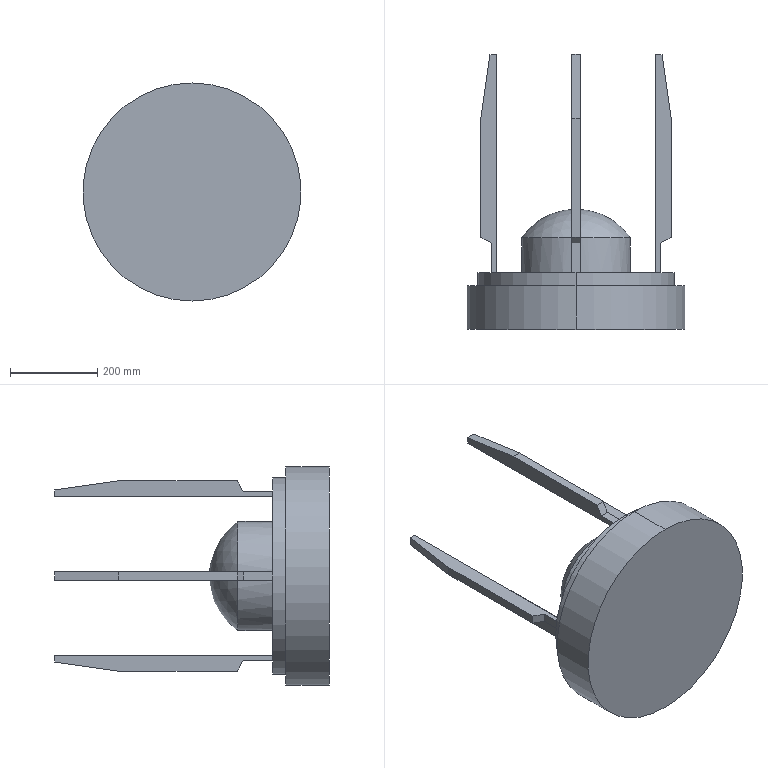Part | SolidWorks | features ICE 3, Revolution 2, CirPattern 1 | 1 solid | 43 faces | box 500 x 630 x 500 mm | volume 31254702 mm3 | plane 35 | cylinder 6 | sphere 2 | commonest cylinder face diameters 250 x2 450 x2 500 x2
STEP:
#1=CARTESIAN_POINT('',(0.,275.519,0.));
#2=VERTEX_POINT('',#1);
#3=CARTESIAN_POINT('',(125.,210.,0.));
#4=VERTEX_POINT('',#3);
#5=CARTESIAN_POINT('',(0.,123.519,0.));
#6=DIRECTION('',(0.,0.,-1.));
#7=DIRECTION('',(-1.,0.,0.));
#8=AXIS2_PLACEMENT_3D('',#5,#6,#7);
#9=CIRCLE('',#8,152.);
#10=EDGE_CURVE('',#2,#4,#9,.T.);
#11=ORIENTED_EDGE('',*,*,#10,.F.);
#12=CARTESIAN_POINT('',(-125.,210.,0.));
#13=VERTEX_POINT('',#12);
#14=CARTESIAN_POINT('',(0.,123.519,0.));
#15=DIRECTION('',(0.,0.,1.));
#16=DIRECTION('',(1.,0.,0.));
#17=AXIS2_PLACEMENT_3D('',#14,#15,#16);
#18=CIRCLE('',#17,152.);
#19=EDGE_CURVE('',#2,#13,#18,.T.);
#20=ORIENTED_EDGE('',*,*,#19,.T.);
#21=CARTESIAN_POINT('',(0.,210.,125.));
#22=VERTEX_POINT('',#21);
#23=CARTESIAN_POINT('',(0.,210.,0.));
#24=DIRECTION('',(0.,1.,0.));
#25=DIRECTION('',(0.,0.,1.));
#26=AXIS2_PLACEMENT_3D('',#23,#24,#25);
#27=CIRCLE('',#26,125.);
#28=EDGE_CURVE('',#13,#22,#27,.T.);
#29=ORIENTED_EDGE('',*,*,#28,.T.);
#30=CARTESIAN_POINT('',(0.,210.,0.));
#31=DIRECTION('',(0.,1.,0.));
#32=DIRECTION('',(0.,0.,1.));
#33=AXIS2_PLACEMENT_3D('',#30,#31,#32);
#34=CIRCLE('',#33,125.);
#35=EDGE_CURVE('',#22,#4,#34,.T.);
#36=ORIENTED_EDGE('',*,*,#35,.T.);
#37=EDGE_LOOP('',(#11,#20,#29,#36));
#38=FACE_OUTER_BOUND('',#37,.T.);
#39=CARTESIAN_POINT('',(0.,123.519,0.));
#40=DIRECTION('',(0.,0.,1.));
#41=DIRECTION('',(1.,0.,0.));
#42=AXIS2_PLACEMENT_3D('',#39,#40,#41);
#43=SPHERICAL_SURFACE('',#42,152.);
#44=ADVANCED_FACE('',(#38),#43,.T.);
#45=ORIENTED_EDGE('',*,*,#35,.F.);
#46=CARTESIAN_POINT('',(0.,130.,125.));
#47=VERTEX_POINT('',#46);
#48=CARTESIAN_POINT('',(0.,210.,125.));
#49=DIRECTION('',(0.,-1.,0.));
#50=VECTOR('',#49,1000.);
#51=LINE('',#48,#50);
#52=EDGE_CURVE('',#22,#47,#51,.T.);
#53=ORIENTED_EDGE('',*,*,#52,.T.);
#54=CARTESIAN_POINT('',(0.,130.,-125.));
#55=VERTEX_POINT('',#54);
#56=CARTESIAN_POINT('',(0.,130.,0.));
#57=DIRECTION('',(0.,1.,0.));
#58=DIRECTION('',(0.,0.,1.));
#59=AXIS2_PLACEMENT_3D('',#56,#57,#58);
#60=CIRCLE('',#59,125.);
#61=EDGE_CURVE('',#47,#55,#60,.T.);
#62=ORIENTED_EDGE('',*,*,#61,.T.);
#63=CARTESIAN_POINT('',(0.,210.,-125.));
#64=VERTEX_POINT('',#63);
#65=CARTESIAN_POINT('',(0.,210.,-125.));
#66=DIRECTION('',(0.,-1.,0.));
#67=VECTOR('',#66,1000.);
#68=LINE('',#65,#67);
#69=EDGE_CURVE('',#64,#55,#68,.T.);
#70=ORIENTED_EDGE('',*,*,#69,.F.);
#71=CARTESIAN_POINT('',(0.,210.,0.));
#72=DIRECTION('',(0.,1.,0.));
#73=DIRECTION('',(0.,0.,1.));
#74=AXIS2_PLACEMENT_3D('',#71,#72,#73);
#75=CIRCLE('',#74,125.);
#76=EDGE_CURVE('',#4,#64,#75,.T.);
#77=ORIENTED_EDGE('',*,*,#76,.F.);
#78=EDGE_LOOP('',(#45,#53,#62,#70,#77));
#79=FACE_OUTER_BOUND('',#78,.T.);
#80=CARTESIAN_POINT('',(0.,210.,0.));
#81=DIRECTION('',(0.,-1.,0.));
#82=DIRECTION('',(0.,0.,-1.));
#83=AXIS2_PLACEMENT_3D('',#80,#81,#82);
#84=CYLINDRICAL_SURFACE('',#83,125.);
#85=ADVANCED_FACE('',(#79),#84,.T.);
#86=CARTESIAN_POINT('',(0.,130.,225.));
#87=VERTEX_POINT('',#86);
#88=CARTESIAN_POINT('',(0.,130.,-225.));
#89=VERTEX_POINT('',#88);
#90=CARTESIAN_POINT('',(0.,130.,0.));
#91=DIRECTION('',(0.,1.,0.));
#92=DIRECTION('',(0.,0.,1.));
#93=AXIS2_PLACEMENT_3D('',#90,#91,#92);
#94=CIRCLE('',#93,225.);
#95=EDGE_CURVE('',#87,#89,#94,.T.);
#96=ORIENTED_EDGE('',*,*,#95,.F.);
#97=CARTESIAN_POINT('',(0.,100.,225.));
#98=VERTEX_POINT('',#97);
#99=CARTESIAN_POINT('',(0.,130.,225.));
#100=DIRECTION('',(0.,-1.,0.));
#101=VECTOR('',#100,1000.);
#102=LINE('',#99,#101);
#103=EDGE_CURVE('',#87,#98,#102,.T.);
#104=ORIENTED_EDGE('',*,*,#103,.T.);
#105=CARTESIAN_POINT('',(0.,100.,-225.));
#106=VERTEX_POINT('',#105);
#107=CARTESIAN_POINT('',(0.,100.,0.));
#108=DIRECTION('',(0.,1.,0.));
#109=DIRECTION('',(0.,0.,1.));
#110=AXIS2_PLACEMENT_3D('',#107,#108,#109);
#111=CIRCLE('',#110,225.);
#112=EDGE_CURVE('',#98,#106,#111,.T.);
#113=ORIENTED_EDGE('',*,*,#112,.T.);
#114=CARTESIAN_POINT('',(0.,130.,-225.));
#115=DIRECTION('',(0.,-1.,0.));
#116=VECTOR('',#115,1000.);
#117=LINE('',#114,#116);
#118=EDGE_CURVE('',#89,#106,#117,.T.);
#119=ORIENTED_EDGE('',*,*,#118,.F.);
#120=EDGE_LOOP('',(#96,#104,#113,#119));
#121=FACE_OUTER_BOUND('',#120,.T.);
#122=CARTESIAN_POINT('',(0.,130.,0.));
#123=DIRECTION('',(0.,-1.,0.));
#124=DIRECTION('',(0.,0.,-1.));
#125=AXIS2_PLACEMENT_3D('',#122,#123,#124);
#126=CYLINDRICAL_SURFACE('',#125,225.);
#127=ADVANCED_FACE('',(#121),#126,.T.);
#128=CARTESIAN_POINT('',(0.,100.,-250.));
#129=VERTEX_POINT('',#128);
#130=CARTESIAN_POINT('',(0.,100.,250.));
#131=VERTEX_POINT('',#130);
#132=CARTESIAN_POINT('',(0.,100.,0.));
#133=DIRECTION('',(0.,-1.,0.));
#134=DIRECTION('',(0.,0.,-1.));
#135=AXIS2_PLACEMENT_3D('',#132,#133,#134);
#136=CIRCLE('',#135,250.);
#137=EDGE_CURVE('',#129,#131,#136,.T.);
#138=ORIENTED_EDGE('',*,*,#137,.T.);
#139=CARTESIAN_POINT('',(0.,0.,250.));
#140=VERTEX_POINT('',#139);
#141=CARTESIAN_POINT('',(0.,0.,250.));
#142=DIRECTION('',(0.,-1.,0.));
#143=VECTOR('',#142,1000.);
#144=LINE('',#141,#143);
#145=EDGE_CURVE('',#131,#140,#144,.T.);
#146=ORIENTED_EDGE('',*,*,#145,.T.);
#147=CARTESIAN_POINT('',(0.,0.,-250.));
#148=VERTEX_POINT('',#147);
#149=CARTESIAN_POINT('',(0.,0.,0.));
#150=DIRECTION('',(0.,-1.,0.));
#151=DIRECTION('',(0.,0.,-1.));
#152=AXIS2_PLACEMENT_3D('',#149,#150,#151);
#153=CIRCLE('',#152,250.);
#154=EDGE_CURVE('',#148,#140,#153,.T.);
#155=ORIENTED_EDGE('',*,*,#154,.F.);
#156=CARTESIAN_POINT('',(0.,0.,-250.));
#157=DIRECTION('',(0.,-1.,0.));
#158=VECTOR('',#157,1000.);
#159=LINE('',#156,#158);
#160=EDGE_CURVE('',#129,#148,#159,.T.);
#161=ORIENTED_EDGE('',*,*,#160,.F.);
#162=EDGE_LOOP('',(#138,#146,#155,#161));
#163=FACE_OUTER_BOUND('',#162,.T.);
#164=CARTESIAN_POINT('',(0.,0.,0.));
#165=DIRECTION('',(0.,-1.,0.));
#166=DIRECTION('',(0.,0.,-1.));
#167=AXIS2_PLACEMENT_3D('',#164,#165,#166);
#168=CYLINDRICAL_SURFACE('',#167,250.);
#169=ADVANCED_FACE('',(#163),#168,.T.);
#170=ORIENTED_EDGE('',*,*,#154,.T.);
#171=CARTESIAN_POINT('',(0.,0.,0.));
#172=DIRECTION('',(0.,-1.,0.));
#173=DIRECTION('',(0.,0.,-1.));
#174=AXIS2_PLACEMENT_3D('',#171,#172,#173);
#175=CIRCLE('',#174,250.);
#176=EDGE_CURVE('',#140,#148,#175,.T.);
#177=ORIENTED_EDGE('',*,*,#176,.T.);
#178=EDGE_LOOP('',(#170,#177));
#179=FACE_OUTER_BOUND('',#178,.T.);
#180=CARTESIAN_POINT('',(250.,0.,0.));
#181=DIRECTION('',(0.,-1.,0.));
#182=DIRECTION('',(0.,0.,-1.));
#183=AXIS2_PLACEMENT_3D('',#180,#181,#182);
#184=PLANE('',#183);
#185=ADVANCED_FACE('',(#179),#184,.T.);
#186=CARTESIAN_POINT('',(0.,100.,0.));
#187=DIRECTION('',(0.,1.,0.));
#188=DIRECTION('',(0.,0.,1.));
#189=AXIS2_PLACEMENT_3D('',#186,#187,#188);
#190=CIRCLE('',#189,225.);
#191=EDGE_CURVE('',#106,#98,#190,.T.);
#192=ORIENTED_EDGE('',*,*,#191,.F.);
#193=ORIENTED_EDGE('',*,*,#112,.F.);
#194=EDGE_LOOP('',(#192,#193));
#195=FACE_BOUND('',#194,.T.);
#196=ORIENTED_EDGE('',*,*,#137,.F.);
#197=CARTESIAN_POINT('',(0.,100.,0.));
#198=DIRECTION('',(0.,-1.,0.));
#199=DIRECTION('',(0.,0.,-1.));
#200=AXIS2_PLACEMENT_3D('',#197,#198,#199);
#201=CIRCLE('',#200,250.);
#202=EDGE_CURVE('',#131,#129,#201,.T.);
#203=ORIENTED_EDGE('',*,*,#202,.F.);
#204=EDGE_LOOP('',(#196,#203));
#205=FACE_OUTER_BOUND('',#204,.T.);
#206=CARTESIAN_POINT('',(0.,100.,0.));
#207=DIRECTION('',(0.,1.,0.));
#208=DIRECTION('',(0.,0.,1.));
#209=AXIS2_PLACEMENT_3D('',#206,#207,#208);
#210=PLANE('',#209);
#211=ADVANCED_FACE('',(#195,#205),#210,.T.);
#212=ORIENTED_EDGE('',*,*,#145,.F.);
#213=ORIENTED_EDGE('',*,*,#202,.T.);
#214=ORIENTED_EDGE('',*,*,#160,.T.);
#215=ORIENTED_EDGE('',*,*,#176,.F.);
#216=EDGE_LOOP('',(#212,#213,#214,#215));
#217=FACE_OUTER_BOUND('',#216,.T.);
#218=CARTESIAN_POINT('',(0.,0.,0.));
#219=DIRECTION('',(0.,-1.,0.));
#220=DIRECTION('',(0.,0.,-1.));
#221=AXIS2_PLACEMENT_3D('',#218,#219,#220);
#222=CYLINDRICAL_SURFACE('',#221,250.);
#223=ADVANCED_FACE('',(#217),#222,.T.);
#224=ORIENTED_EDGE('',*,*,#103,.F.);
#225=CARTESIAN_POINT('',(0.,130.,0.));
#226=DIRECTION('',(0.,1.,0.));
#227=DIRECTION('',(0.,0.,1.));
#228=AXIS2_PLACEMENT_3D('',#225,#226,#227);
#229=CIRCLE('',#228,225.);
#230=EDGE_CURVE('',#89,#87,#229,.T.);
#231=ORIENTED_EDGE('',*,*,#230,.F.);
#232=ORIENTED_EDGE('',*,*,#118,.T.);
#233=ORIENTED_EDGE('',*,*,#191,.T.);
#234=EDGE_LOOP('',(#224,#231,#232,#233));
#235=FACE_OUTER_BOUND('',#234,.T.);
#236=CARTESIAN_POINT('',(0.,130.,0.));
#237=DIRECTION('',(0.,-1.,0.));
#238=DIRECTION('',(0.,0.,-1.));
#239=AXIS2_PLACEMENT_3D('',#236,#237,#238);
#240=CYLINDRICAL_SURFACE('',#239,225.);
#241=ADVANCED_FACE('',(#235),#240,.T.);
#242=CARTESIAN_POINT('',(-10.,130.,-194.003));
#243=VERTEX_POINT('',#242);
#244=CARTESIAN_POINT('',(-10.,130.,-182.358));
#245=VERTEX_POINT('',#244);
#246=CARTESIAN_POINT('',(-10.,130.,-194.003));
#247=DIRECTION('',(0.,0.,1.));
#248=VECTOR('',#247,1000.);
#249=LINE('',#246,#248);
#250=EDGE_CURVE('',#243,#245,#249,.T.);
#251=ORIENTED_EDGE('',*,*,#250,.F.);
#252=CARTESIAN_POINT('',(10.,130.,-194.003));
#253=VERTEX_POINT('',#252);
#254=CARTESIAN_POINT('',(-10.,130.,-194.003));
#255=DIRECTION('',(1.,0.,0.));
#256=VECTOR('',#255,1000.);
#257=LINE('',#254,#256);
#258=EDGE_CURVE('',#243,#253,#257,.T.);
#259=ORIENTED_EDGE('',*,*,#258,.T.);
#260=CARTESIAN_POINT('',(10.,130.,-182.358));
#261=VERTEX_POINT('',#260);
#262=CARTESIAN_POINT('',(10.,130.,-194.003));
#263=DIRECTION('',(0.,0.,1.));
#264=VECTOR('',#263,1000.);
#265=LINE('',#262,#264);
#266=EDGE_CURVE('',#253,#261,#265,.T.);
#267=ORIENTED_EDGE('',*,*,#266,.T.);
#268=CARTESIAN_POINT('',(-10.,130.,-182.358));
#269=DIRECTION('',(1.,0.,0.));
#270=VECTOR('',#269,1000.);
#271=LINE('',#268,#270);
#272=EDGE_CURVE('',#245,#261,#271,.T.);
#273=ORIENTED_EDGE('',*,*,#272,.F.);
#274=EDGE_LOOP('',(#251,#259,#267,#273));
#275=FACE_BOUND('',#274,.T.);
#276=CARTESIAN_POINT('',(194.003,130.,-10.));
#277=VERTEX_POINT('',#276);
#278=CARTESIAN_POINT('',(182.358,130.,-10.));
#279=VERTEX_POINT('',#278);
#280=CARTESIAN_POINT('',(194.003,130.,-10.));
#281=DIRECTION('',(-1.,0.,0.));
#282=VECTOR('',#281,1000.);
#283=LINE('',#280,#282);
#284=EDGE_CURVE('',#277,#279,#283,.T.);
#285=ORIENTED_EDGE('',*,*,#284,.F.);
#286=CARTESIAN_POINT('',(194.003,130.,10.));
#287=VERTEX_POINT('',#286);
#288=CARTESIAN_POINT('',(194.003,130.,-10.));
#289=DIRECTION('',(0.,0.,1.));
#290=VECTOR('',#289,1000.);
#291=LINE('',#288,#290);
#292=EDGE_CURVE('',#277,#287,#291,.T.);
#293=ORIENTED_EDGE('',*,*,#292,.T.);
#294=CARTESIAN_POINT('',(182.358,130.,10.));
#295=VERTEX_POINT('',#294);
#296=CARTESIAN_POINT('',(194.003,130.,10.));
#297=DIRECTION('',(-1.,0.,0.));
#298=VECTOR('',#297,1000.);
#299=LINE('',#296,#298);
#300=EDGE_CURVE('',#287,#295,#299,.T.);
#301=ORIENTED_EDGE('',*,*,#300,.T.);
#302=CARTESIAN_POINT('',(182.358,130.,-10.));
#303=DIRECTION('',(0.,0.,1.));
#304=VECTOR('',#303,1000.);
#305=LINE('',#302,#304);
#306=EDGE_CURVE('',#279,#295,#305,.T.);
#307=ORIENTED_EDGE('',*,*,#306,.F.);
#308=EDGE_LOOP('',(#285,#293,#301,#307));
#309=FACE_BOUND('',#308,.T.);
#310=CARTESIAN_POINT('',(10.,130.,194.003));
#311=VERTEX_POINT('',#310);
#312=CARTESIAN_POINT('',(10.,130.,182.358));
#313=VERTEX_POINT('',#312);
#314=CARTESIAN_POINT('',(10.,130.,194.003));
#315=DIRECTION('',(0.,0.,-1.));
#316=VECTOR('',#315,1000.);
#317=LINE('',#314,#316);
#318=EDGE_CURVE('',#311,#313,#317,.T.);
#319=ORIENTED_EDGE('',*,*,#318,.F.);
#320=CARTESIAN_POINT('',(-10.,130.,194.003));
#321=VERTEX_POINT('',#320);
#322=CARTESIAN_POINT('',(10.,130.,194.003));
#323=DIRECTION('',(-1.,0.,0.));
#324=VECTOR('',#323,1000.);
#325=LINE('',#322,#324);
#326=EDGE_CURVE('',#311,#321,#325,.T.);
#327=ORIENTED_EDGE('',*,*,#326,.T.);
#328=CARTESIAN_POINT('',(-10.,130.,182.358));
#329=VERTEX_POINT('',#328);
#330=CARTESIAN_POINT('',(-10.,130.,194.003));
#331=DIRECTION('',(0.,0.,-1.));
#332=VECTOR('',#331,1000.);
#333=LINE('',#330,#332);
#334=EDGE_CURVE('',#321,#329,#333,.T.);
#335=ORIENTED_EDGE('',*,*,#334,.T.);
#336=CARTESIAN_POINT('',(10.,130.,182.358));
#337=DIRECTION('',(-1.,0.,0.));
#338=VECTOR('',#337,1000.);
#339=LINE('',#336,#338);
#340=EDGE_CURVE('',#313,#329,#339,.T.);
#341=ORIENTED_EDGE('',*,*,#340,.F.);
#342=EDGE_LOOP('',(#319,#327,#335,#341));
#343=FACE_BOUND('',#342,.T.);
#344=CARTESIAN_POINT('',(-194.003,130.,10.));
#345=VERTEX_POINT('',#344);
#346=CARTESIAN_POINT('',(-182.358,130.,10.));
#347=VERTEX_POINT('',#346);
#348=CARTESIAN_POINT('',(-194.003,130.,10.));
#349=DIRECTION('',(1.,0.,0.));
#350=VECTOR('',#349,1000.);
#351=LINE('',#348,#350);
#352=EDGE_CURVE('',#345,#347,#351,.T.);
#353=ORIENTED_EDGE('',*,*,#352,.F.);
#354=CARTESIAN_POINT('',(-194.003,130.,-10.));
#355=VERTEX_POINT('',#354);
#356=CARTESIAN_POINT('',(-194.003,130.,10.));
#357=DIRECTION('',(0.,0.,-1.));
#358=VECTOR('',#357,1000.);
#359=LINE('',#356,#358);
#360=EDGE_CURVE('',#345,#355,#359,.T.);
#361=ORIENTED_EDGE('',*,*,#360,.T.);
#362=CARTESIAN_POINT('',(-182.358,130.,-10.));
#363=VERTEX_POINT('',#362);
#364=CARTESIAN_POINT('',(-194.003,130.,-10.));
#365=DIRECTION('',(1.,0.,0.));
#366=VECTOR('',#365,1000.);
#367=LINE('',#364,#366);
#368=EDGE_CURVE('',#355,#363,#367,.T.);
#369=ORIENTED_EDGE('',*,*,#368,.T.);
#370=CARTESIAN_POINT('',(-182.358,130.,10.));
#371=DIRECTION('',(0.,0.,-1.));
#372=VECTOR('',#371,1000.);
#373=LINE('',#370,#372);
#374=EDGE_CURVE('',#347,#363,#373,.T.);
#375=ORIENTED_EDGE('',*,*,#374,.F.);
#376=EDGE_LOOP('',(#353,#361,#369,#375));
#377=FACE_BOUND('',#376,.T.);
#378=CARTESIAN_POINT('',(0.,130.,0.));
#379=DIRECTION('',(0.,1.,0.));
#380=DIRECTION('',(0.,0.,1.));
#381=AXIS2_PLACEMENT_3D('',#378,#379,#380);
#382=CIRCLE('',#381,125.);
#383=EDGE_CURVE('',#55,#47,#382,.T.);
#384=ORIENTED_EDGE('',*,*,#383,.F.);
#385=ORIENTED_EDGE('',*,*,#61,.F.);
#386=EDGE_LOOP('',(#384,#385));
#387=FACE_BOUND('',#386,.T.);
#388=ORIENTED_EDGE('',*,*,#230,.T.);
#389=ORIENTED_EDGE('',*,*,#95,.T.);
#390=EDGE_LOOP('',(#388,#389));
#391=FACE_OUTER_BOUND('',#390,.T.);
#392=CARTESIAN_POINT('',(0.,130.,0.));
#393=DIRECTION('',(0.,1.,0.));
#394=DIRECTION('',(0.,0.,1.));
#395=AXIS2_PLACEMENT_3D('',#392,#393,#394);
#396=PLANE('',#395);
#397=ADVANCED_FACE('',(#275,#309,#343,#377,#387,#391),#396,.T.);
#398=ORIENTED_EDGE('',*,*,#52,.F.);
#399=ORIENTED_EDGE('',*,*,#28,.F.);
#400=CARTESIAN_POINT('',(0.,210.,0.));
#401=DIRECTION('',(0.,1.,0.));
#402=DIRECTION('',(0.,0.,1.));
#403=AXIS2_PLACEMENT_3D('',#400,#401,#402);
#404=CIRCLE('',#403,125.);
#405=EDGE_CURVE('',#64,#13,#404,.T.);
#406=ORIENTED_EDGE('',*,*,#405,.F.);
#407=ORIENTED_EDGE('',*,*,#69,.T.);
#408=ORIENTED_EDGE('',*,*,#383,.T.);
#409=EDGE_LOOP('',(#398,#399,#406,#407,#408));
#410=FACE_OUTER_BOUND('',#409,.T.);
#411=CARTESIAN_POINT('',(0.,210.,0.));
#412=DIRECTION('',(0.,-1.,0.));
#413=DIRECTION('',(0.,0.,-1.));
#414=AXIS2_PLACEMENT_3D('',#411,#412,#413);
#415=CYLINDRICAL_SURFACE('',#414,125.);
#416=ADVANCED_FACE('',(#410),#415,.T.);
#417=ORIENTED_EDGE('',*,*,#19,.F.);
#418=ORIENTED_EDGE('',*,*,#10,.T.);
#419=ORIENTED_EDGE('',*,*,#76,.T.);
#420=ORIENTED_EDGE('',*,*,#405,.T.);
#421=EDGE_LOOP('',(#417,#418,#419,#420));
#422=FACE_OUTER_BOUND('',#421,.T.);
#423=CARTESIAN_POINT('',(0.,123.519,0.));
#424=DIRECTION('',(0.,0.,1.));
#425=DIRECTION('',(1.,0.,0.));
#426=AXIS2_PLACEMENT_3D('',#423,#424,#425);
#427=SPHERICAL_SURFACE('',#426,152.);
#428=ADVANCED_FACE('',(#422),#427,.T.);
#429=CARTESIAN_POINT('',(-194.003,197.687,-10.));
#430=VERTEX_POINT('',#429);
#431=CARTESIAN_POINT('',(-194.003,130.,-10.));
#432=DIRECTION('',(0.,-1.,0.));
#433=VECTOR('',#432,1000.);
#434=LINE('',#431,#433);
#435=EDGE_CURVE('',#430,#355,#434,.T.);
#436=ORIENTED_EDGE('',*,*,#435,.T.);
#437=ORIENTED_EDGE('',*,*,#360,.F.);
#438=CARTESIAN_POINT('',(-194.003,197.687,10.));
#439=VERTEX_POINT('',#438);
#440=CARTESIAN_POINT('',(-194.003,130.,10.));
#441=DIRECTION('',(0.,-1.,0.));
#442=VECTOR('',#441,1000.);
#443=LINE('',#440,#442);
#444=EDGE_CURVE('',#439,#345,#443,.T.);
#445=ORIENTED_EDGE('',*,*,#444,.F.);
#446=CARTESIAN_POINT('',(-194.003,197.687,10.));
#447=DIRECTION('',(0.,0.,-1.));
#448=VECTOR('',#447,1000.);
#449=LINE('',#446,#448);
#450=EDGE_CURVE('',#439,#430,#449,.T.);
#451=ORIENTED_EDGE('',*,*,#450,.T.);
#452=EDGE_LOOP('',(#436,#437,#445,#451));
#453=FACE_OUTER_BOUND('',#452,.T.);
#454=CARTESIAN_POINT('',(-194.003,130.,10.));
#455=DIRECTION('',(1.,0.,0.));
#456=DIRECTION('',(0.,1.,0.));
#457=AXIS2_PLACEMENT_3D('',#454,#455,#456);
#458=PLANE('',#457);
#459=ADVANCED_FACE('',(#453),#458,.F.);
#460=CARTESIAN_POINT('',(-182.358,630.,-10.));
#461=VERTEX_POINT('',#460);
#462=CARTESIAN_POINT('',(-182.358,145.263,-10.));
#463=DIRECTION('',(0.,1.,0.));
#464=VECTOR('',#463,1000.);
#465=LINE('',#462,#464);
#466=EDGE_CURVE('',#363,#461,#465,.T.);
#467=ORIENTED_EDGE('',*,*,#466,.T.);
#468=CARTESIAN_POINT('',(-182.358,630.,10.));
#469=VERTEX_POINT('',#468);
#470=CARTESIAN_POINT('',(-182.358,630.,10.));
#471=DIRECTION('',(0.,0.,-1.));
#472=VECTOR('',#471,1000.);
#473=LINE('',#470,#472);
#474=EDGE_CURVE('',#469,#461,#473,.T.);
#475=ORIENTED_EDGE('',*,*,#474,.F.);
#476=CARTESIAN_POINT('',(-182.358,130.,10.));
#477=DIRECTION('',(0.,1.,0.));
#478=VECTOR('',#477,1000.);
#479=LINE('',#476,#478);
#480=EDGE_CURVE('',#347,#469,#479,.T.);
#481=ORIENTED_EDGE('',*,*,#480,.F.);
#482=ORIENTED_EDGE('',*,*,#374,.T.);
#483=EDGE_LOOP('',(#467,#475,#481,#482));
#484=FACE_OUTER_BOUND('',#483,.T.);
#485=CARTESIAN_POINT('',(-182.358,145.263,10.));
#486=DIRECTION('',(-1.,0.,0.));
#487=DIRECTION('',(0.,0.,1.));
#488=AXIS2_PLACEMENT_3D('',#485,#486,#487);
#489=PLANE('',#488);
#490=ADVANCED_FACE('',(#484),#489,.F.);
#491=CARTESIAN_POINT('',(-197.365,630.,-10.));
#492=VERTEX_POINT('',#491);
#493=CARTESIAN_POINT('',(-182.358,630.,-10.));
#494=DIRECTION('',(-1.,0.,0.));
#495=VECTOR('',#494,1000.);
#496=LINE('',#493,#495);
#497=EDGE_CURVE('',#461,#492,#496,.T.);
#498=ORIENTED_EDGE('',*,*,#497,.T.);
#499=CARTESIAN_POINT('',(-197.365,630.,10.));
#500=VERTEX_POINT('',#499);
#501=CARTESIAN_POINT('',(-197.365,630.,10.));
#502=DIRECTION('',(0.,0.,-1.));
#503=VECTOR('',#502,1000.);
#504=LINE('',#501,#503);
#505=EDGE_CURVE('',#500,#492,#504,.T.);
#506=ORIENTED_EDGE('',*,*,#505,.F.);
#507=CARTESIAN_POINT('',(-182.358,630.,10.));
#508=DIRECTION('',(-1.,0.,0.));
#509=VECTOR('',#508,1000.);
#510=LINE('',#507,#509);
#511=EDGE_CURVE('',#469,#500,#510,.T.);
#512=ORIENTED_EDGE('',*,*,#511,.F.);
#513=ORIENTED_EDGE('',*,*,#474,.T.);
#514=EDGE_LOOP('',(#498,#506,#512,#513));
#515=FACE_OUTER_BOUND('',#514,.T.);
#516=CARTESIAN_POINT('',(-182.358,630.,10.));
#517=DIRECTION('',(0.,-1.,0.));
#518=DIRECTION('',(0.,0.,-1.));
#519=AXIS2_PLACEMENT_3D('',#516,#517,#518);
#520=PLANE('',#519);
#521=ADVANCED_FACE('',(#515),#520,.F.);
#522=CARTESIAN_POINT('',(-218.162,483.058,-10.));
#523=VERTEX_POINT('',#522);
#524=CARTESIAN_POINT('',(-197.365,630.,-10.));
#525=DIRECTION('',(-0.1401,-0.9901,0.));
#526=VECTOR('',#525,1000.);
#527=LINE('',#524,#526);
#528=EDGE_CURVE('',#492,#523,#527,.T.);
#529=ORIENTED_EDGE('',*,*,#528,.T.);
#530=CARTESIAN_POINT('',(-218.162,483.058,10.));
#531=VERTEX_POINT('',#530);
#532=CARTESIAN_POINT('',(-218.162,483.058,10.));
#533=DIRECTION('',(0.,0.,-1.));
#534=VECTOR('',#533,1000.);
#535=LINE('',#532,#534);
#536=EDGE_CURVE('',#531,#523,#535,.T.);
#537=ORIENTED_EDGE('',*,*,#536,.F.);
#538=CARTESIAN_POINT('',(-197.365,630.,10.));
#539=DIRECTION('',(-0.1401,-0.9901,0.));
#540=VECTOR('',#539,1000.);
#541=LINE('',#538,#540);
#542=EDGE_CURVE('',#500,#531,#541,.T.);
#543=ORIENTED_EDGE('',*,*,#542,.F.);
#544=ORIENTED_EDGE('',*,*,#505,.T.);
#545=EDGE_LOOP('',(#529,#537,#543,#544));
#546=FACE_OUTER_BOUND('',#545,.T.);
#547=CARTESIAN_POINT('',(-197.365,630.,10.));
#548=DIRECTION('',(0.9901,-0.1401,0.));
#549=DIRECTION('',(0.1401,0.9901,0.));
#550=AXIS2_PLACEMENT_3D('',#547,#548,#549);
#551=PLANE('',#550);
#552=ADVANCED_FACE('',(#546),#551,.F.);
#553=CARTESIAN_POINT('',(-218.162,211.102,-10.));
#554=VERTEX_POINT('',#553);
#555=CARTESIAN_POINT('',(-218.162,483.058,-10.));
#556=DIRECTION('',(0.,-1.,0.));
#557=VECTOR('',#556,1000.);
#558=LINE('',#555,#557);
#559=EDGE_CURVE('',#523,#554,#558,.T.);
#560=ORIENTED_EDGE('',*,*,#559,.T.);
#561=CARTESIAN_POINT('',(-218.162,211.102,10.));
#562=VERTEX_POINT('',#561);
#563=CARTESIAN_POINT('',(-218.162,211.102,10.));
#564=DIRECTION('',(0.,0.,-1.));
#565=VECTOR('',#564,1000.);
#566=LINE('',#563,#565);
#567=EDGE_CURVE('',#562,#554,#566,.T.);
#568=ORIENTED_EDGE('',*,*,#567,.F.);
#569=CARTESIAN_POINT('',(-218.162,483.058,10.));
#570=DIRECTION('',(0.,-1.,0.));
#571=VECTOR('',#570,1000.);
#572=LINE('',#569,#571);
#573=EDGE_CURVE('',#531,#562,#572,.T.);
#574=ORIENTED_EDGE('',*,*,#573,.F.);
#575=ORIENTED_EDGE('',*,*,#536,.T.);
#576=EDGE_LOOP('',(#560,#568,#574,#575));
#577=FACE_OUTER_BOUND('',#576,.T.);
#578=CARTESIAN_POINT('',(-218.162,483.058,10.));
#579=DIRECTION('',(1.,0.,0.));
#580=DIRECTION('',(0.,1.,0.));
#581=AXIS2_PLACEMENT_3D('',#578,#579,#580);
#582=PLANE('',#581);
#583=ADVANCED_FACE('',(#577),#582,.F.);
#584=CARTESIAN_POINT('',(-218.162,211.102,-10.));
#585=DIRECTION('',(0.8743,-0.4855,0.));
#586=VECTOR('',#585,1000.);
#587=LINE('',#584,#586);
#588=EDGE_CURVE('',#554,#430,#587,.T.);
#589=ORIENTED_EDGE('',*,*,#588,.T.);
#590=ORIENTED_EDGE('',*,*,#450,.F.);
#591=CARTESIAN_POINT('',(-218.162,211.102,10.));
#592=DIRECTION('',(0.8743,-0.4855,0.));
#593=VECTOR('',#592,1000.);
#594=LINE('',#591,#593);
#595=EDGE_CURVE('',#562,#439,#594,.T.);
#596=ORIENTED_EDGE('',*,*,#595,.F.);
#597=ORIENTED_EDGE('',*,*,#567,.T.);
#598=EDGE_LOOP('',(#589,#590,#596,#597));
#599=FACE_OUTER_BOUND('',#598,.T.);
#600=CARTESIAN_POINT('',(-218.162,211.102,10.));
#601=DIRECTION('',(0.4855,0.8743,0.));
#602=DIRECTION('',(-0.8743,0.4855,0.));
#603=AXIS2_PLACEMENT_3D('',#600,#601,#602);
#604=PLANE('',#603);
#605=ADVANCED_FACE('',(#599),#604,.F.);
#606=ORIENTED_EDGE('',*,*,#444,.T.);
#607=ORIENTED_EDGE('',*,*,#352,.T.);
#608=ORIENTED_EDGE('',*,*,#480,.T.);
#609=ORIENTED_EDGE('',*,*,#511,.T.);
#610=ORIENTED_EDGE('',*,*,#542,.T.);
#611=ORIENTED_EDGE('',*,*,#573,.T.);
#612=ORIENTED_EDGE('',*,*,#595,.T.);
#613=EDGE_LOOP('',(#606,#607,#608,#609,#610,#611,#612));
#614=FACE_OUTER_BOUND('',#613,.T.);
#615=CARTESIAN_POINT('',(0.,0.,10.));
#616=DIRECTION('',(0.,0.,1.));
#617=DIRECTION('',(1.,0.,0.));
#618=AXIS2_PLACEMENT_3D('',#615,#616,#617);
#619=PLANE('',#618);
#620=ADVANCED_FACE('',(#614),#619,.T.);
#621=ORIENTED_EDGE('',*,*,#435,.F.);
#622=ORIENTED_EDGE('',*,*,#588,.F.);
#623=ORIENTED_EDGE('',*,*,#559,.F.);
#624=ORIENTED_EDGE('',*,*,#528,.F.);
#625=ORIENTED_EDGE('',*,*,#497,.F.);
#626=ORIENTED_EDGE('',*,*,#466,.F.);
#627=ORIENTED_EDGE('',*,*,#368,.F.);
#628=EDGE_LOOP('',(#621,#622,#623,#624,#625,#626,#627));
#629=FACE_OUTER_BOUND('',#628,.T.);
#630=CARTESIAN_POINT('',(0.,0.,-10.));
#631=DIRECTION('',(0.,0.,1.));
#632=DIRECTION('',(1.,0.,0.));
#633=AXIS2_PLACEMENT_3D('',#630,#631,#632);
#634=PLANE('',#633);
#635=ADVANCED_FACE('',(#629),#634,.F.);
#636=CARTESIAN_POINT('',(-10.,197.687,194.003));
#637=VERTEX_POINT('',#636);
#638=CARTESIAN_POINT('',(-10.,130.,194.003));
#639=DIRECTION('',(0.,-1.,0.));
#640=VECTOR('',#639,1000.);
#641=LINE('',#638,#640);
#642=EDGE_CURVE('',#637,#321,#641,.T.);
#643=ORIENTED_EDGE('',*,*,#642,.T.);
#644=ORIENTED_EDGE('',*,*,#326,.F.);
#645=CARTESIAN_POINT('',(10.,197.687,194.003));
#646=VERTEX_POINT('',#645);
#647=CARTESIAN_POINT('',(10.,130.,194.003));
#648=DIRECTION('',(0.,-1.,0.));
#649=VECTOR('',#648,1000.);
#650=LINE('',#647,#649);
#651=EDGE_CURVE('',#646,#311,#650,.T.);
#652=ORIENTED_EDGE('',*,*,#651,.F.);
#653=CARTESIAN_POINT('',(10.,197.687,194.003));
#654=DIRECTION('',(-1.,0.,0.));
#655=VECTOR('',#654,1000.);
#656=LINE('',#653,#655);
#657=EDGE_CURVE('',#646,#637,#656,.T.);
#658=ORIENTED_EDGE('',*,*,#657,.T.);
#659=EDGE_LOOP('',(#643,#644,#652,#658));
#660=FACE_OUTER_BOUND('',#659,.T.);
#661=CARTESIAN_POINT('',(10.,130.,194.003));
#662=DIRECTION('',(0.,0.,-1.));
#663=DIRECTION('',(-1.,0.,0.));
#664=AXIS2_PLACEMENT_3D('',#661,#662,#663);
#665=PLANE('',#664);
#666=ADVANCED_FACE('',(#660),#665,.F.);
#667=CARTESIAN_POINT('',(-10.,630.,182.358));
#668=VERTEX_POINT('',#667);
#669=CARTESIAN_POINT('',(-10.,145.263,182.358));
#670=DIRECTION('',(0.,1.,0.));
#671=VECTOR('',#670,1000.);
#672=LINE('',#669,#671);
#673=EDGE_CURVE('',#329,#668,#672,.T.);
#674=ORIENTED_EDGE('',*,*,#673,.T.);
#675=CARTESIAN_POINT('',(10.,630.,182.358));
#676=VERTEX_POINT('',#675);
#677=CARTESIAN_POINT('',(10.,630.,182.358));
#678=DIRECTION('',(-1.,0.,0.));
#679=VECTOR('',#678,1000.);
#680=LINE('',#677,#679);
#681=EDGE_CURVE('',#676,#668,#680,.T.);
#682=ORIENTED_EDGE('',*,*,#681,.F.);
#683=CARTESIAN_POINT('',(10.,130.,182.358));
#684=DIRECTION('',(0.,1.,0.));
#685=VECTOR('',#684,1000.);
#686=LINE('',#683,#685);
#687=EDGE_CURVE('',#313,#676,#686,.T.);
#688=ORIENTED_EDGE('',*,*,#687,.F.);
#689=ORIENTED_EDGE('',*,*,#340,.T.);
#690=EDGE_LOOP('',(#674,#682,#688,#689));
#691=FACE_OUTER_BOUND('',#690,.T.);
#692=CARTESIAN_POINT('',(10.,145.263,182.358));
#693=DIRECTION('',(0.,0.,1.));
#694=DIRECTION('',(1.,0.,0.));
#695=AXIS2_PLACEMENT_3D('',#692,#693,#694);
#696=PLANE('',#695);
#697=ADVANCED_FACE('',(#691),#696,.F.);
#698=CARTESIAN_POINT('',(-10.,630.,197.365));
#699=VERTEX_POINT('',#698);
#700=CARTESIAN_POINT('',(-10.,630.,182.358));
#701=DIRECTION('',(0.,0.,1.));
#702=VECTOR('',#701,1000.);
#703=LINE('',#700,#702);
#704=EDGE_CURVE('',#668,#699,#703,.T.);
#705=ORIENTED_EDGE('',*,*,#704,.T.);
#706=CARTESIAN_POINT('',(10.,630.,197.365));
#707=VERTEX_POINT('',#706);
#708=CARTESIAN_POINT('',(10.,630.,197.365));
#709=DIRECTION('',(-1.,0.,0.));
#710=VECTOR('',#709,1000.);
#711=LINE('',#708,#710);
#712=EDGE_CURVE('',#707,#699,#711,.T.);
#713=ORIENTED_EDGE('',*,*,#712,.F.);
#714=CARTESIAN_POINT('',(10.,630.,182.358));
#715=DIRECTION('',(0.,0.,1.));
#716=VECTOR('',#715,1000.);
#717=LINE('',#714,#716);
#718=EDGE_CURVE('',#676,#707,#717,.T.);
#719=ORIENTED_EDGE('',*,*,#718,.F.);
#720=ORIENTED_EDGE('',*,*,#681,.T.);
#721=EDGE_LOOP('',(#705,#713,#719,#720));
#722=FACE_OUTER_BOUND('',#721,.T.);
#723=CARTESIAN_POINT('',(10.,630.,182.358));
#724=DIRECTION('',(0.,-1.,0.));
#725=DIRECTION('',(0.,0.,-1.));
#726=AXIS2_PLACEMENT_3D('',#723,#724,#725);
#727=PLANE('',#726);
#728=ADVANCED_FACE('',(#722),#727,.F.);
#729=CARTESIAN_POINT('',(-10.,483.058,218.162));
#730=VERTEX_POINT('',#729);
#731=CARTESIAN_POINT('',(-10.,630.,197.365));
#732=DIRECTION('',(0.,-0.9901,0.1401));
#733=VECTOR('',#732,1000.);
#734=LINE('',#731,#733);
#735=EDGE_CURVE('',#699,#730,#734,.T.);
#736=ORIENTED_EDGE('',*,*,#735,.T.);
#737=CARTESIAN_POINT('',(10.,483.058,218.162));
#738=VERTEX_POINT('',#737);
#739=CARTESIAN_POINT('',(10.,483.058,218.162));
#740=DIRECTION('',(-1.,0.,0.));
#741=VECTOR('',#740,1000.);
#742=LINE('',#739,#741);
#743=EDGE_CURVE('',#738,#730,#742,.T.);
#744=ORIENTED_EDGE('',*,*,#743,.F.);
#745=CARTESIAN_POINT('',(10.,630.,197.365));
#746=DIRECTION('',(0.,-0.9901,0.1401));
#747=VECTOR('',#746,1000.);
#748=LINE('',#745,#747);
#749=EDGE_CURVE('',#707,#738,#748,.T.);
#750=ORIENTED_EDGE('',*,*,#749,.F.);
#751=ORIENTED_EDGE('',*,*,#712,.T.);
#752=EDGE_LOOP('',(#736,#744,#750,#751));
#753=FACE_OUTER_BOUND('',#752,.T.);
#754=CARTESIAN_POINT('',(10.,630.,197.365));
#755=DIRECTION('',(0.,-0.1401,-0.9901));
#756=DIRECTION('',(0.,0.9901,-0.1401));
#757=AXIS2_PLACEMENT_3D('',#754,#755,#756);
#758=PLANE('',#757);
#759=ADVANCED_FACE('',(#753),#758,.F.);
#760=CARTESIAN_POINT('',(-10.,211.102,218.162));
#761=VERTEX_POINT('',#760);
#762=CARTESIAN_POINT('',(-10.,483.058,218.162));
#763=DIRECTION('',(0.,-1.,0.));
#764=VECTOR('',#763,1000.);
#765=LINE('',#762,#764);
#766=EDGE_CURVE('',#730,#761,#765,.T.);
#767=ORIENTED_EDGE('',*,*,#766,.T.);
#768=CARTESIAN_POINT('',(10.,211.102,218.162));
#769=VERTEX_POINT('',#768);
#770=CARTESIAN_POINT('',(10.,211.102,218.162));
#771=DIRECTION('',(-1.,0.,0.));
#772=VECTOR('',#771,1000.);
#773=LINE('',#770,#772);
#774=EDGE_CURVE('',#769,#761,#773,.T.);
#775=ORIENTED_EDGE('',*,*,#774,.F.);
#776=CARTESIAN_POINT('',(10.,483.058,218.162));
#777=DIRECTION('',(0.,-1.,0.));
#778=VECTOR('',#777,1000.);
#779=LINE('',#776,#778);
#780=EDGE_CURVE('',#738,#769,#779,.T.);
#781=ORIENTED_EDGE('',*,*,#780,.F.);
#782=ORIENTED_EDGE('',*,*,#743,.T.);
#783=EDGE_LOOP('',(#767,#775,#781,#782));
#784=FACE_OUTER_BOUND('',#783,.T.);
#785=CARTESIAN_POINT('',(10.,483.058,218.162));
#786=DIRECTION('',(0.,0.,-1.));
#787=DIRECTION('',(-1.,0.,0.));
#788=AXIS2_PLACEMENT_3D('',#785,#786,#787);
#789=PLANE('',#788);
#790=ADVANCED_FACE('',(#784),#789,.F.);
#791=CARTESIAN_POINT('',(-10.,211.102,218.162));
#792=DIRECTION('',(0.,-0.4855,-0.8743));
#793=VECTOR('',#792,1000.);
#794=LINE('',#791,#793);
#795=EDGE_CURVE('',#761,#637,#794,.T.);
#796=ORIENTED_EDGE('',*,*,#795,.T.);
#797=ORIENTED_EDGE('',*,*,#657,.F.);
#798=CARTESIAN_POINT('',(10.,211.102,218.162));
#799=DIRECTION('',(0.,-0.4855,-0.8743));
#800=VECTOR('',#799,1000.);
#801=LINE('',#798,#800);
#802=EDGE_CURVE('',#769,#646,#801,.T.);
#803=ORIENTED_EDGE('',*,*,#802,.F.);
#804=ORIENTED_EDGE('',*,*,#774,.T.);
#805=EDGE_LOOP('',(#796,#797,#803,#804));
#806=FACE_OUTER_BOUND('',#805,.T.);
#807=CARTESIAN_POINT('',(10.,211.102,218.162));
#808=DIRECTION('',(0.,0.8743,-0.4855));
#809=DIRECTION('',(0.,0.4855,0.8743));
#810=AXIS2_PLACEMENT_3D('',#807,#808,#809);
#811=PLANE('',#810);
#812=ADVANCED_FACE('',(#806),#811,.F.);
#813=ORIENTED_EDGE('',*,*,#651,.T.);
#814=ORIENTED_EDGE('',*,*,#318,.T.);
#815=ORIENTED_EDGE('',*,*,#687,.T.);
#816=ORIENTED_EDGE('',*,*,#718,.T.);
#817=ORIENTED_EDGE('',*,*,#749,.T.);
#818=ORIENTED_EDGE('',*,*,#780,.T.);
#819=ORIENTED_EDGE('',*,*,#802,.T.);
#820=EDGE_LOOP('',(#813,#814,#815,#816,#817,#818,#819));
#821=FACE_OUTER_BOUND('',#820,.T.);
#822=CARTESIAN_POINT('',(10.,0.,0.));
#823=DIRECTION('',(1.,0.,0.));
#824=DIRECTION('',(0.,0.,-1.));
#825=AXIS2_PLACEMENT_3D('',#822,#823,#824);
#826=PLANE('',#825);
#827=ADVANCED_FACE('',(#821),#826,.T.);
#828=ORIENTED_EDGE('',*,*,#642,.F.);
#829=ORIENTED_EDGE('',*,*,#795,.F.);
#830=ORIENTED_EDGE('',*,*,#766,.F.);
#831=ORIENTED_EDGE('',*,*,#735,.F.);
#832=ORIENTED_EDGE('',*,*,#704,.F.);
#833=ORIENTED_EDGE('',*,*,#673,.F.);
#834=ORIENTED_EDGE('',*,*,#334,.F.);
#835=EDGE_LOOP('',(#828,#829,#830,#831,#832,#833,#834));
#836=FACE_OUTER_BOUND('',#835,.T.);
#837=CARTESIAN_POINT('',(-10.,0.,0.));
#838=DIRECTION('',(1.,0.,0.));
#839=DIRECTION('',(0.,0.,-1.));
#840=AXIS2_PLACEMENT_3D('',#837,#838,#839);
#841=PLANE('',#840);
#842=ADVANCED_FACE('',(#836),#841,.F.);
#843=CARTESIAN_POINT('',(194.003,197.687,10.));
#844=VERTEX_POINT('',#843);
#845=CARTESIAN_POINT('',(194.003,130.,10.));
#846=DIRECTION('',(0.,-1.,0.));
#847=VECTOR('',#846,1000.);
#848=LINE('',#845,#847);
#849=EDGE_CURVE('',#844,#287,#848,.T.);
#850=ORIENTED_EDGE('',*,*,#849,.T.);
#851=ORIENTED_EDGE('',*,*,#292,.F.);
#852=CARTESIAN_POINT('',(194.003,197.687,-10.));
#853=VERTEX_POINT('',#852);
#854=CARTESIAN_POINT('',(194.003,130.,-10.));
#855=DIRECTION('',(0.,-1.,0.));
#856=VECTOR('',#855,1000.);
#857=LINE('',#854,#856);
#858=EDGE_CURVE('',#853,#277,#857,.T.);
#859=ORIENTED_EDGE('',*,*,#858,.F.);
#860=CARTESIAN_POINT('',(194.003,197.687,-10.));
#861=DIRECTION('',(0.,0.,1.));
#862=VECTOR('',#861,1000.);
#863=LINE('',#860,#862);
#864=EDGE_CURVE('',#853,#844,#863,.T.);
#865=ORIENTED_EDGE('',*,*,#864,.T.);
#866=EDGE_LOOP('',(#850,#851,#859,#865));
#867=FACE_OUTER_BOUND('',#866,.T.);
#868=CARTESIAN_POINT('',(194.003,130.,-10.));
#869=DIRECTION('',(-1.,0.,0.));
#870=DIRECTION('',(0.,-1.,0.));
#871=AXIS2_PLACEMENT_3D('',#868,#869,#870);
#872=PLANE('',#871);
#873=ADVANCED_FACE('',(#867),#872,.F.);
#874=CARTESIAN_POINT('',(182.358,630.,10.));
#875=VERTEX_POINT('',#874);
#876=CARTESIAN_POINT('',(182.358,145.263,10.));
#877=DIRECTION('',(0.,1.,0.));
#878=VECTOR('',#877,1000.);
#879=LINE('',#876,#878);
#880=EDGE_CURVE('',#295,#875,#879,.T.);
#881=ORIENTED_EDGE('',*,*,#880,.T.);
#882=CARTESIAN_POINT('',(182.358,630.,-10.));
#883=VERTEX_POINT('',#882);
#884=CARTESIAN_POINT('',(182.358,630.,-10.));
#885=DIRECTION('',(0.,0.,1.));
#886=VECTOR('',#885,1000.);
#887=LINE('',#884,#886);
#888=EDGE_CURVE('',#883,#875,#887,.T.);
#889=ORIENTED_EDGE('',*,*,#888,.F.);
#890=CARTESIAN_POINT('',(182.358,130.,-10.));
#891=DIRECTION('',(0.,1.,0.));
#892=VECTOR('',#891,1000.);
#893=LINE('',#890,#892);
#894=EDGE_CURVE('',#279,#883,#893,.T.);
#895=ORIENTED_EDGE('',*,*,#894,.F.);
#896=ORIENTED_EDGE('',*,*,#306,.T.);
#897=EDGE_LOOP('',(#881,#889,#895,#896));
#898=FACE_OUTER_BOUND('',#897,.T.);
#899=CARTESIAN_POINT('',(182.358,145.263,-10.));
#900=DIRECTION('',(1.,0.,0.));
#901=DIRECTION('',(0.,0.,-1.));
#902=AXIS2_PLACEMENT_3D('',#899,#900,#901);
#903=PLANE('',#902);
#904=ADVANCED_FACE('',(#898),#903,.F.);
#905=CARTESIAN_POINT('',(197.365,630.,10.));
#906=VERTEX_POINT('',#905);
#907=CARTESIAN_POINT('',(182.358,630.,10.));
#908=DIRECTION('',(1.,0.,0.));
#909=VECTOR('',#908,1000.);
#910=LINE('',#907,#909);
#911=EDGE_CURVE('',#875,#906,#910,.T.);
#912=ORIENTED_EDGE('',*,*,#911,.T.);
#913=CARTESIAN_POINT('',(197.365,630.,-10.));
#914=VERTEX_POINT('',#913);
#915=CARTESIAN_POINT('',(197.365,630.,-10.));
#916=DIRECTION('',(0.,0.,1.));
#917=VECTOR('',#916,1000.);
#918=LINE('',#915,#917);
#919=EDGE_CURVE('',#914,#906,#918,.T.);
#920=ORIENTED_EDGE('',*,*,#919,.F.);
#921=CARTESIAN_POINT('',(182.358,630.,-10.));
#922=DIRECTION('',(1.,0.,0.));
#923=VECTOR('',#922,1000.);
#924=LINE('',#921,#923);
#925=EDGE_CURVE('',#883,#914,#924,.T.);
#926=ORIENTED_EDGE('',*,*,#925,.F.);
#927=ORIENTED_EDGE('',*,*,#888,.T.);
#928=EDGE_LOOP('',(#912,#920,#926,#927));
#929=FACE_OUTER_BOUND('',#928,.T.);
#930=CARTESIAN_POINT('',(182.358,630.,-10.));
#931=DIRECTION('',(0.,-1.,0.));
#932=DIRECTION('',(0.,0.,-1.));
#933=AXIS2_PLACEMENT_3D('',#930,#931,#932);
#934=PLANE('',#933);
#935=ADVANCED_FACE('',(#929),#934,.F.);
#936=CARTESIAN_POINT('',(218.162,483.058,10.));
#937=VERTEX_POINT('',#936);
#938=CARTESIAN_POINT('',(197.365,630.,10.));
#939=DIRECTION('',(0.1401,-0.9901,0.));
#940=VECTOR('',#939,1000.);
#941=LINE('',#938,#940);
#942=EDGE_CURVE('',#906,#937,#941,.T.);
#943=ORIENTED_EDGE('',*,*,#942,.T.);
#944=CARTESIAN_POINT('',(218.162,483.058,-10.));
#945=VERTEX_POINT('',#944);
#946=CARTESIAN_POINT('',(218.162,483.058,-10.));
#947=DIRECTION('',(0.,0.,1.));
#948=VECTOR('',#947,1000.);
#949=LINE('',#946,#948);
#950=EDGE_CURVE('',#945,#937,#949,.T.);
#951=ORIENTED_EDGE('',*,*,#950,.F.);
#952=CARTESIAN_POINT('',(197.365,630.,-10.));
#953=DIRECTION('',(0.1401,-0.9901,0.));
#954=VECTOR('',#953,1000.);
#955=LINE('',#952,#954);
#956=EDGE_CURVE('',#914,#945,#955,.T.);
#957=ORIENTED_EDGE('',*,*,#956,.F.);
#958=ORIENTED_EDGE('',*,*,#919,.T.);
#959=EDGE_LOOP('',(#943,#951,#957,#958));
#960=FACE_OUTER_BOUND('',#959,.T.);
#961=CARTESIAN_POINT('',(197.365,630.,-10.));
#962=DIRECTION('',(-0.9901,-0.1401,0.));
#963=DIRECTION('',(0.1401,-0.9901,0.));
#964=AXIS2_PLACEMENT_3D('',#961,#962,#963);
#965=PLANE('',#964);
#966=ADVANCED_FACE('',(#960),#965,.F.);
#967=CARTESIAN_POINT('',(218.162,211.102,10.));
#968=VERTEX_POINT('',#967);
#969=CARTESIAN_POINT('',(218.162,483.058,10.));
#970=DIRECTION('',(0.,-1.,0.));
#971=VECTOR('',#970,1000.);
#972=LINE('',#969,#971);
#973=EDGE_CURVE('',#937,#968,#972,.T.);
#974=ORIENTED_EDGE('',*,*,#973,.T.);
#975=CARTESIAN_POINT('',(218.162,211.102,-10.));
#976=VERTEX_POINT('',#975);
#977=CARTESIAN_POINT('',(218.162,211.102,-10.));
#978=DIRECTION('',(0.,0.,1.));
#979=VECTOR('',#978,1000.);
#980=LINE('',#977,#979);
#981=EDGE_CURVE('',#976,#968,#980,.T.);
#982=ORIENTED_EDGE('',*,*,#981,.F.);
#983=CARTESIAN_POINT('',(218.162,483.058,-10.));
#984=DIRECTION('',(0.,-1.,0.));
#985=VECTOR('',#984,1000.);
#986=LINE('',#983,#985);
#987=EDGE_CURVE('',#945,#976,#986,.T.);
#988=ORIENTED_EDGE('',*,*,#987,.F.);
#989=ORIENTED_EDGE('',*,*,#950,.T.);
#990=EDGE_LOOP('',(#974,#982,#988,#989));
#991=FACE_OUTER_BOUND('',#990,.T.);
#992=CARTESIAN_POINT('',(218.162,483.058,-10.));
#993=DIRECTION('',(-1.,0.,0.));
#994=DIRECTION('',(0.,-1.,0.));
#995=AXIS2_PLACEMENT_3D('',#992,#993,#994);
#996=PLANE('',#995);
#997=ADVANCED_FACE('',(#991),#996,.F.);
#998=CARTESIAN_POINT('',(218.162,211.102,10.));
#999=DIRECTION('',(-0.8743,-0.4855,0.));
#1000=VECTOR('',#999,1000.);
#1001=LINE('',#998,#1000);
#1002=EDGE_CURVE('',#968,#844,#1001,.T.);
#1003=ORIENTED_EDGE('',*,*,#1002,.T.);
#1004=ORIENTED_EDGE('',*,*,#864,.F.);
#1005=CARTESIAN_POINT('',(218.162,211.102,-10.));
#1006=DIRECTION('',(-0.8743,-0.4855,0.));
#1007=VECTOR('',#1006,1000.);
#1008=LINE('',#1005,#1007);
#1009=EDGE_CURVE('',#976,#853,#1008,.T.);
#1010=ORIENTED_EDGE('',*,*,#1009,.F.);
#1011=ORIENTED_EDGE('',*,*,#981,.T.);
#1012=EDGE_LOOP('',(#1003,#1004,#1010,#1011));
#1013=FACE_OUTER_BOUND('',#1012,.T.);
#1014=CARTESIAN_POINT('',(218.162,211.102,-10.));
#1015=DIRECTION('',(-0.4855,0.8743,0.));
#1016=DIRECTION('',(-0.8743,-0.4855,0.));
#1017=AXIS2_PLACEMENT_3D('',#1014,#1015,#1016);
#1018=PLANE('',#1017);
#1019=ADVANCED_FACE('',(#1013),#1018,.F.);
#1020=ORIENTED_EDGE('',*,*,#858,.T.);
#1021=ORIENTED_EDGE('',*,*,#284,.T.);
#1022=ORIENTED_EDGE('',*,*,#894,.T.);
#1023=ORIENTED_EDGE('',*,*,#925,.T.);
#1024=ORIENTED_EDGE('',*,*,#956,.T.);
#1025=ORIENTED_EDGE('',*,*,#987,.T.);
#1026=ORIENTED_EDGE('',*,*,#1009,.T.);
#1027=EDGE_LOOP('',(#1020,#1021,#1022,#1023,#1024,#1025,#1026));
#1028=FACE_OUTER_BOUND('',#1027,.T.);
#1029=CARTESIAN_POINT('',(0.,0.,-10.));
#1030=DIRECTION('',(0.,0.,-1.));
#1031=DIRECTION('',(-1.,0.,0.));
#1032=AXIS2_PLACEMENT_3D('',#1029,#1030,#1031);
#1033=PLANE('',#1032);
#1034=ADVANCED_FACE('',(#1028),#1033,.T.);
#1035=ORIENTED_EDGE('',*,*,#849,.F.);
#1036=ORIENTED_EDGE('',*,*,#1002,.F.);
#1037=ORIENTED_EDGE('',*,*,#973,.F.);
#1038=ORIENTED_EDGE('',*,*,#942,.F.);
#1039=ORIENTED_EDGE('',*,*,#911,.F.);
#1040=ORIENTED_EDGE('',*,*,#880,.F.);
#1041=ORIENTED_EDGE('',*,*,#300,.F.);
#1042=EDGE_LOOP('',(#1035,#1036,#1037,#1038,#1039,#1040,#1041));
#1043=FACE_OUTER_BOUND('',#1042,.T.);
#1044=CARTESIAN_POINT('',(0.,0.,10.));
#1045=DIRECTION('',(0.,0.,-1.));
#1046=DIRECTION('',(-1.,0.,0.));
#1047=AXIS2_PLACEMENT_3D('',#1044,#1045,#1046);
#1048=PLANE('',#1047);
#1049=ADVANCED_FACE('',(#1043),#1048,.F.);
#1050=CARTESIAN_POINT('',(10.,197.687,-194.003));
#1051=VERTEX_POINT('',#1050);
#1052=CARTESIAN_POINT('',(10.,130.,-194.003));
#1053=DIRECTION('',(0.,-1.,0.));
#1054=VECTOR('',#1053,1000.);
#1055=LINE('',#1052,#1054);
#1056=EDGE_CURVE('',#1051,#253,#1055,.T.);
#1057=ORIENTED_EDGE('',*,*,#1056,.T.);
#1058=ORIENTED_EDGE('',*,*,#258,.F.);
#1059=CARTESIAN_POINT('',(-10.,197.687,-194.003));
#1060=VERTEX_POINT('',#1059);
#1061=CARTESIAN_POINT('',(-10.,130.,-194.003));
#1062=DIRECTION('',(0.,-1.,0.));
#1063=VECTOR('',#1062,1000.);
#1064=LINE('',#1061,#1063);
#1065=EDGE_CURVE('',#1060,#243,#1064,.T.);
#1066=ORIENTED_EDGE('',*,*,#1065,.F.);
#1067=CARTESIAN_POINT('',(-10.,197.687,-194.003));
#1068=DIRECTION('',(1.,0.,0.));
#1069=VECTOR('',#1068,1000.);
#1070=LINE('',#1067,#1069);
#1071=EDGE_CURVE('',#1060,#1051,#1070,.T.);
#1072=ORIENTED_EDGE('',*,*,#1071,.T.);
#1073=EDGE_LOOP('',(#1057,#1058,#1066,#1072));
#1074=FACE_OUTER_BOUND('',#1073,.T.);
#1075=CARTESIAN_POINT('',(-10.,130.,-194.003));
#1076=DIRECTION('',(0.,0.,1.));
#1077=DIRECTION('',(1.,0.,0.));
#1078=AXIS2_PLACEMENT_3D('',#1075,#1076,#1077);
#1079=PLANE('',#1078);
#1080=ADVANCED_FACE('',(#1074),#1079,.F.);
#1081=CARTESIAN_POINT('',(10.,630.,-182.358));
#1082=VERTEX_POINT('',#1081);
#1083=CARTESIAN_POINT('',(10.,145.263,-182.358));
#1084=DIRECTION('',(0.,1.,0.));
#1085=VECTOR('',#1084,1000.);
#1086=LINE('',#1083,#1085);
#1087=EDGE_CURVE('',#261,#1082,#1086,.T.);
#1088=ORIENTED_EDGE('',*,*,#1087,.T.);
#1089=CARTESIAN_POINT('',(-10.,630.,-182.358));
#1090=VERTEX_POINT('',#1089);
#1091=CARTESIAN_POINT('',(-10.,630.,-182.358));
#1092=DIRECTION('',(1.,0.,0.));
#1093=VECTOR('',#1092,1000.);
#1094=LINE('',#1091,#1093);
#1095=EDGE_CURVE('',#1090,#1082,#1094,.T.);
#1096=ORIENTED_EDGE('',*,*,#1095,.F.);
#1097=CARTESIAN_POINT('',(-10.,130.,-182.358));
#1098=DIRECTION('',(0.,1.,0.));
#1099=VECTOR('',#1098,1000.);
#1100=LINE('',#1097,#1099);
#1101=EDGE_CURVE('',#245,#1090,#1100,.T.);
#1102=ORIENTED_EDGE('',*,*,#1101,.F.);
#1103=ORIENTED_EDGE('',*,*,#272,.T.);
#1104=EDGE_LOOP('',(#1088,#1096,#1102,#1103));
#1105=FACE_OUTER_BOUND('',#1104,.T.);
#1106=CARTESIAN_POINT('',(-10.,145.263,-182.358));
#1107=DIRECTION('',(0.,0.,-1.));
#1108=DIRECTION('',(-1.,0.,0.));
#1109=AXIS2_PLACEMENT_3D('',#1106,#1107,#1108);
#1110=PLANE('',#1109);
#1111=ADVANCED_FACE('',(#1105),#1110,.F.);
#1112=CARTESIAN_POINT('',(10.,630.,-197.365));
#1113=VERTEX_POINT('',#1112);
#1114=CARTESIAN_POINT('',(10.,630.,-182.358));
#1115=DIRECTION('',(0.,0.,-1.));
#1116=VECTOR('',#1115,1000.);
#1117=LINE('',#1114,#1116);
#1118=EDGE_CURVE('',#1082,#1113,#1117,.T.);
#1119=ORIENTED_EDGE('',*,*,#1118,.T.);
#1120=CARTESIAN_POINT('',(-10.,630.,-197.365));
#1121=VERTEX_POINT('',#1120);
#1122=CARTESIAN_POINT('',(-10.,630.,-197.365));
#1123=DIRECTION('',(1.,0.,0.));
#1124=VECTOR('',#1123,1000.);
#1125=LINE('',#1122,#1124);
#1126=EDGE_CURVE('',#1121,#1113,#1125,.T.);
#1127=ORIENTED_EDGE('',*,*,#1126,.F.);
#1128=CARTESIAN_POINT('',(-10.,630.,-182.358));
#1129=DIRECTION('',(0.,0.,-1.));
#1130=VECTOR('',#1129,1000.);
#1131=LINE('',#1128,#1130);
#1132=EDGE_CURVE('',#1090,#1121,#1131,.T.);
#1133=ORIENTED_EDGE('',*,*,#1132,.F.);
#1134=ORIENTED_EDGE('',*,*,#1095,.T.);
#1135=EDGE_LOOP('',(#1119,#1127,#1133,#1134));
#1136=FACE_OUTER_BOUND('',#1135,.T.);
#1137=CARTESIAN_POINT('',(-10.,630.,-182.358));
#1138=DIRECTION('',(0.,-1.,0.));
#1139=DIRECTION('',(0.,0.,-1.));
#1140=AXIS2_PLACEMENT_3D('',#1137,#1138,#1139);
#1141=PLANE('',#1140);
#1142=ADVANCED_FACE('',(#1136),#1141,.F.);
#1143=CARTESIAN_POINT('',(10.,483.058,-218.162));
#1144=VERTEX_POINT('',#1143);
#1145=CARTESIAN_POINT('',(10.,630.,-197.365));
#1146=DIRECTION('',(0.,-0.9901,-0.1401));
#1147=VECTOR('',#1146,1000.);
#1148=LINE('',#1145,#1147);
#1149=EDGE_CURVE('',#1113,#1144,#1148,.T.);
#1150=ORIENTED_EDGE('',*,*,#1149,.T.);
#1151=CARTESIAN_POINT('',(-10.,483.058,-218.162));
#1152=VERTEX_POINT('',#1151);
#1153=CARTESIAN_POINT('',(-10.,483.058,-218.162));
#1154=DIRECTION('',(1.,0.,0.));
#1155=VECTOR('',#1154,1000.);
#1156=LINE('',#1153,#1155);
#1157=EDGE_CURVE('',#1152,#1144,#1156,.T.);
#1158=ORIENTED_EDGE('',*,*,#1157,.F.);
#1159=CARTESIAN_POINT('',(-10.,630.,-197.365));
#1160=DIRECTION('',(0.,-0.9901,-0.1401));
#1161=VECTOR('',#1160,1000.);
#1162=LINE('',#1159,#1161);
#1163=EDGE_CURVE('',#1121,#1152,#1162,.T.);
#1164=ORIENTED_EDGE('',*,*,#1163,.F.);
#1165=ORIENTED_EDGE('',*,*,#1126,.T.);
#1166=EDGE_LOOP('',(#1150,#1158,#1164,#1165));
#1167=FACE_OUTER_BOUND('',#1166,.T.);
#1168=CARTESIAN_POINT('',(-10.,630.,-197.365));
#1169=DIRECTION('',(0.,-0.1401,0.9901));
#1170=DIRECTION('',(0.,-0.9901,-0.1401));
#1171=AXIS2_PLACEMENT_3D('',#1168,#1169,#1170);
#1172=PLANE('',#1171);
#1173=ADVANCED_FACE('',(#1167),#1172,.F.);
#1174=CARTESIAN_POINT('',(10.,211.102,-218.162));
#1175=VERTEX_POINT('',#1174);
#1176=CARTESIAN_POINT('',(10.,483.058,-218.162));
#1177=DIRECTION('',(0.,-1.,0.));
#1178=VECTOR('',#1177,1000.);
#1179=LINE('',#1176,#1178);
#1180=EDGE_CURVE('',#1144,#1175,#1179,.T.);
#1181=ORIENTED_EDGE('',*,*,#1180,.T.);
#1182=CARTESIAN_POINT('',(-10.,211.102,-218.162));
#1183=VERTEX_POINT('',#1182);
#1184=CARTESIAN_POINT('',(-10.,211.102,-218.162));
#1185=DIRECTION('',(1.,0.,0.));
#1186=VECTOR('',#1185,1000.);
#1187=LINE('',#1184,#1186);
#1188=EDGE_CURVE('',#1183,#1175,#1187,.T.);
#1189=ORIENTED_EDGE('',*,*,#1188,.F.);
#1190=CARTESIAN_POINT('',(-10.,483.058,-218.162));
#1191=DIRECTION('',(0.,-1.,0.));
#1192=VECTOR('',#1191,1000.);
#1193=LINE('',#1190,#1192);
#1194=EDGE_CURVE('',#1152,#1183,#1193,.T.);
#1195=ORIENTED_EDGE('',*,*,#1194,.F.);
#1196=ORIENTED_EDGE('',*,*,#1157,.T.);
#1197=EDGE_LOOP('',(#1181,#1189,#1195,#1196));
#1198=FACE_OUTER_BOUND('',#1197,.T.);
#1199=CARTESIAN_POINT('',(-10.,483.058,-218.162));
#1200=DIRECTION('',(0.,0.,1.));
#1201=DIRECTION('',(1.,0.,0.));
#1202=AXIS2_PLACEMENT_3D('',#1199,#1200,#1201);
#1203=PLANE('',#1202);
#1204=ADVANCED_FACE('',(#1198),#1203,.F.);
#1205=CARTESIAN_POINT('',(10.,211.102,-218.162));
#1206=DIRECTION('',(0.,-0.4855,0.8743));
#1207=VECTOR('',#1206,1000.);
#1208=LINE('',#1205,#1207);
#1209=EDGE_CURVE('',#1175,#1051,#1208,.T.);
#1210=ORIENTED_EDGE('',*,*,#1209,.T.);
#1211=ORIENTED_EDGE('',*,*,#1071,.F.);
#1212=CARTESIAN_POINT('',(-10.,211.102,-218.162));
#1213=DIRECTION('',(0.,-0.4855,0.8743));
#1214=VECTOR('',#1213,1000.);
#1215=LINE('',#1212,#1214);
#1216=EDGE_CURVE('',#1183,#1060,#1215,.T.);
#1217=ORIENTED_EDGE('',*,*,#1216,.F.);
#1218=ORIENTED_EDGE('',*,*,#1188,.T.);
#1219=EDGE_LOOP('',(#1210,#1211,#1217,#1218));
#1220=FACE_OUTER_BOUND('',#1219,.T.);
#1221=CARTESIAN_POINT('',(-10.,211.102,-218.162));
#1222=DIRECTION('',(0.,0.8743,0.4855));
#1223=DIRECTION('',(0.,-0.4855,0.8743));
#1224=AXIS2_PLACEMENT_3D('',#1221,#1222,#1223);
#1225=PLANE('',#1224);
#1226=ADVANCED_FACE('',(#1220),#1225,.F.);
#1227=ORIENTED_EDGE('',*,*,#1065,.T.);
#1228=ORIENTED_EDGE('',*,*,#250,.T.);
#1229=ORIENTED_EDGE('',*,*,#1101,.T.);
#1230=ORIENTED_EDGE('',*,*,#1132,.T.);
#1231=ORIENTED_EDGE('',*,*,#1163,.T.);
#1232=ORIENTED_EDGE('',*,*,#1194,.T.);
#1233=ORIENTED_EDGE('',*,*,#1216,.T.);
#1234=EDGE_LOOP('',(#1227,#1228,#1229,#1230,#1231,#1232,#1233));
#1235=FACE_OUTER_BOUND('',#1234,.T.);
#1236=CARTESIAN_POINT('',(-10.,0.,0.));
#1237=DIRECTION('',(-1.,0.,0.));
#1238=DIRECTION('',(0.,0.,1.));
#1239=AXIS2_PLACEMENT_3D('',#1236,#1237,#1238);
#1240=PLANE('',#1239);
#1241=ADVANCED_FACE('',(#1235),#1240,.T.);
#1242=ORIENTED_EDGE('',*,*,#1056,.F.);
#1243=ORIENTED_EDGE('',*,*,#1209,.F.);
#1244=ORIENTED_EDGE('',*,*,#1180,.F.);
#1245=ORIENTED_EDGE('',*,*,#1149,.F.);
#1246=ORIENTED_EDGE('',*,*,#1118,.F.);
#1247=ORIENTED_EDGE('',*,*,#1087,.F.);
#1248=ORIENTED_EDGE('',*,*,#266,.F.);
#1249=EDGE_LOOP('',(#1242,#1243,#1244,#1245,#1246,#1247,#1248));
#1250=FACE_OUTER_BOUND('',#1249,.T.);
#1251=CARTESIAN_POINT('',(10.,0.,0.));
#1252=DIRECTION('',(-1.,0.,0.));
#1253=DIRECTION('',(0.,0.,1.));
#1254=AXIS2_PLACEMENT_3D('',#1251,#1252,#1253);
#1255=PLANE('',#1254);
#1256=ADVANCED_FACE('',(#1250),#1255,.F.);
#1257=CLOSED_SHELL('',(#44,#85,#127,#169,#185,#211,#223,#241,#397,#416,#428,#459,#490,#521,#552,#583,#605,#620,#635,#666,#697,#728,#759,#790,#812,#827,#842,#873,#904,#935,#966,#997,#1019,#1034,#1049,#1080,#1111,#1142,#1173,#1204,#1226,#1241,#1256));
#1258=MANIFOLD_SOLID_BREP('',#1257);
#1259=CARTESIAN_POINT('',(0.,0.,0.));
#1260=DIRECTION('',(0.,0.,1.));
#1261=DIRECTION('',(1.,0.,0.));
#1262=AXIS2_PLACEMENT_3D('',#1259,#1260,#1261);
#1263=(LENGTH_UNIT()NAMED_UNIT(*)SI_UNIT(.MILLI.,.METRE.));
#1264=UNCERTAINTY_MEASURE_WITH_UNIT(LENGTH_MEASURE(0.00001),#1263,'','');
#1265=(NAMED_UNIT(*)PLANE_ANGLE_UNIT()SI_UNIT($,.RADIAN.));
#1266=(NAMED_UNIT(*)SI_UNIT($,.STERADIAN.)SOLID_ANGLE_UNIT());
#1267=(GEOMETRIC_REPRESENTATION_CONTEXT(3)GLOBAL_UNCERTAINTY_ASSIGNED_CONTEXT((#1264))GLOBAL_UNIT_ASSIGNED_CONTEXT((#1263,#1265,#1266))REPRESENTATION_CONTEXT('',''));
#1268=ADVANCED_BREP_SHAPE_REPRESENTATION('',(#1258,#1262),#1267);